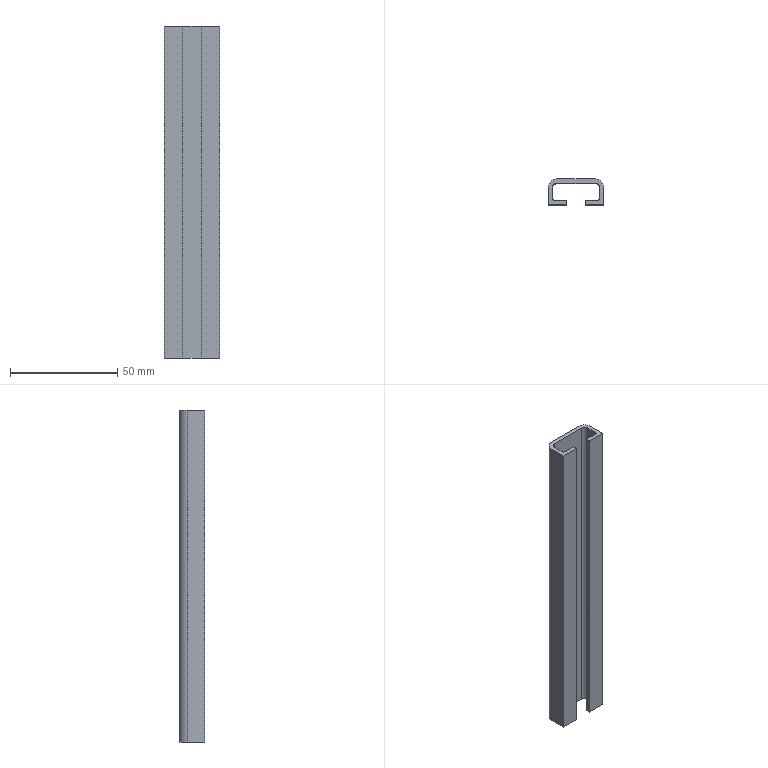Part | STEP file | V00-000000446 | 1 solid | 20 faces | box 26 x 12 x 155 mm | volume 17713 mm3 | plane 14 | cylinder 6 | commonest cylinder face diameters 2 x2 4 x2 8 x2
STEP:
#1=CARTESIAN_POINT('',(-4.25,0.,0.));
#2=VERTEX_POINT('',#1);
#3=CARTESIAN_POINT('',(-4.25,2.,0.));
#4=VERTEX_POINT('',#3);
#5=CARTESIAN_POINT('',(-4.25,1.,0.));
#6=DIRECTION('',(0.,1.,0.));
#7=VECTOR('',#6,1.);
#8=LINE('',#5,#7);
#9=EDGE_CURVE('',#2,#4,#8,.T.);
#10=ORIENTED_EDGE('',*,*,#9,.T.);
#11=CARTESIAN_POINT('',(-4.25,2.,155.));
#12=VERTEX_POINT('',#11);
#13=CARTESIAN_POINT('',(-4.25,2.,77.5));
#14=DIRECTION('',(0.,0.,-1.));
#15=VECTOR('',#14,1.);
#16=LINE('',#13,#15);
#17=EDGE_CURVE('',#12,#4,#16,.T.);
#18=ORIENTED_EDGE('',*,*,#17,.F.);
#19=CARTESIAN_POINT('',(-4.25,0.,155.));
#20=VERTEX_POINT('',#19);
#21=CARTESIAN_POINT('',(-4.25,1.,155.));
#22=DIRECTION('',(0.,1.,0.));
#23=VECTOR('',#22,1.);
#24=LINE('',#21,#23);
#25=EDGE_CURVE('',#20,#12,#24,.T.);
#26=ORIENTED_EDGE('',*,*,#25,.F.);
#27=CARTESIAN_POINT('',(-4.25,0.,77.5));
#28=DIRECTION('',(0.,0.,-1.));
#29=VECTOR('',#28,1.);
#30=LINE('',#27,#29);
#31=EDGE_CURVE('',#20,#2,#30,.T.);
#32=ORIENTED_EDGE('',*,*,#31,.T.);
#33=EDGE_LOOP('',(#10,#18,#26,#32));
#34=FACE_OUTER_BOUND('',#33,.T.);
#35=CARTESIAN_POINT('',(-4.25,2.,155.));
#36=DIRECTION('',(-1.,0.,0.));
#37=DIRECTION('',(0.,0.,1.));
#38=AXIS2_PLACEMENT_3D('',#35,#36,#37);
#39=PLANE('',#38);
#40=ADVANCED_FACE('',(#34),#39,.F.);
#41=ORIENTED_EDGE('',*,*,#9,.F.);
#42=CARTESIAN_POINT('',(-13.,0.,0.));
#43=VERTEX_POINT('',#42);
#44=CARTESIAN_POINT('',(-8.625,0.,0.));
#45=DIRECTION('',(1.,0.,0.));
#46=VECTOR('',#45,1.);
#47=LINE('',#44,#46);
#48=EDGE_CURVE('',#43,#2,#47,.T.);
#49=ORIENTED_EDGE('',*,*,#48,.F.);
#50=CARTESIAN_POINT('',(-13.,8.,0.));
#51=VERTEX_POINT('',#50);
#52=CARTESIAN_POINT('',(-13.,4.,0.));
#53=DIRECTION('',(0.,-1.,0.));
#54=VECTOR('',#53,1.);
#55=LINE('',#52,#54);
#56=EDGE_CURVE('',#51,#43,#55,.T.);
#57=ORIENTED_EDGE('',*,*,#56,.F.);
#58=CARTESIAN_POINT('',(-9.,12.,0.));
#59=VERTEX_POINT('',#58);
#60=CARTESIAN_POINT('',(-9.,8.,0.));
#61=DIRECTION('',(0.,0.,1.));
#62=AXIS2_PLACEMENT_3D('',#60,#61,$);
#63=CIRCLE('',#62,4.);
#64=EDGE_CURVE('',#59,#51,#63,.T.);
#65=ORIENTED_EDGE('',*,*,#64,.F.);
#66=CARTESIAN_POINT('',(9.,12.,0.));
#67=VERTEX_POINT('',#66);
#68=CARTESIAN_POINT('',(0.,12.,0.));
#69=DIRECTION('',(-1.,0.,0.));
#70=VECTOR('',#69,1.);
#71=LINE('',#68,#70);
#72=EDGE_CURVE('',#67,#59,#71,.T.);
#73=ORIENTED_EDGE('',*,*,#72,.F.);
#74=CARTESIAN_POINT('',(13.,8.,0.));
#75=VERTEX_POINT('',#74);
#76=CARTESIAN_POINT('',(9.,8.,0.));
#77=DIRECTION('',(0.,0.,1.));
#78=AXIS2_PLACEMENT_3D('',#76,#77,$);
#79=CIRCLE('',#78,4.);
#80=EDGE_CURVE('',#75,#67,#79,.T.);
#81=ORIENTED_EDGE('',*,*,#80,.F.);
#82=CARTESIAN_POINT('',(13.,0.,0.));
#83=VERTEX_POINT('',#82);
#84=CARTESIAN_POINT('',(13.,4.,0.));
#85=DIRECTION('',(0.,1.,0.));
#86=VECTOR('',#85,1.);
#87=LINE('',#84,#86);
#88=EDGE_CURVE('',#83,#75,#87,.T.);
#89=ORIENTED_EDGE('',*,*,#88,.F.);
#90=CARTESIAN_POINT('',(4.25,0.,0.));
#91=VERTEX_POINT('',#90);
#92=CARTESIAN_POINT('',(8.625,0.,0.));
#93=DIRECTION('',(1.,0.,0.));
#94=VECTOR('',#93,1.);
#95=LINE('',#92,#94);
#96=EDGE_CURVE('',#91,#83,#95,.T.);
#97=ORIENTED_EDGE('',*,*,#96,.F.);
#98=CARTESIAN_POINT('',(4.25,2.,0.));
#99=VERTEX_POINT('',#98);
#100=CARTESIAN_POINT('',(4.25,1.,0.));
#101=DIRECTION('',(0.,-1.,0.));
#102=VECTOR('',#101,1.);
#103=LINE('',#100,#102);
#104=EDGE_CURVE('',#99,#91,#103,.T.);
#105=ORIENTED_EDGE('',*,*,#104,.F.);
#106=CARTESIAN_POINT('',(10.,2.,0.));
#107=VERTEX_POINT('',#106);
#108=CARTESIAN_POINT('',(7.125,2.,0.));
#109=DIRECTION('',(-1.,0.,0.));
#110=VECTOR('',#109,1.);
#111=LINE('',#108,#110);
#112=EDGE_CURVE('',#107,#99,#111,.T.);
#113=ORIENTED_EDGE('',*,*,#112,.F.);
#114=CARTESIAN_POINT('',(11.,3.,0.));
#115=VERTEX_POINT('',#114);
#116=CARTESIAN_POINT('',(10.,3.,0.));
#117=DIRECTION('',(0.,0.,1.));
#118=AXIS2_PLACEMENT_3D('',#116,#117,$);
#119=CIRCLE('',#118,1.);
#120=EDGE_CURVE('',#107,#115,#119,.T.);
#121=ORIENTED_EDGE('',*,*,#120,.T.);
#122=CARTESIAN_POINT('',(11.,8.,0.));
#123=VERTEX_POINT('',#122);
#124=CARTESIAN_POINT('',(11.,5.5,0.));
#125=DIRECTION('',(0.,-1.,0.));
#126=VECTOR('',#125,1.);
#127=LINE('',#124,#126);
#128=EDGE_CURVE('',#123,#115,#127,.T.);
#129=ORIENTED_EDGE('',*,*,#128,.F.);
#130=CARTESIAN_POINT('',(9.,10.,0.));
#131=VERTEX_POINT('',#130);
#132=CARTESIAN_POINT('',(9.,10.,0.));
#133=CARTESIAN_POINT('',(9.208,10.,0.));
#134=CARTESIAN_POINT('',(9.416,9.973,0.));
#135=CARTESIAN_POINT('',(9.619,9.919,0.));
#136=CARTESIAN_POINT('',(10.006,9.759,0.));
#137=CARTESIAN_POINT('',(10.341,9.506,0.));
#138=CARTESIAN_POINT('',(10.49,9.358,0.));
#139=CARTESIAN_POINT('',(10.747,9.027,0.));
#140=CARTESIAN_POINT('',(10.911,8.642,0.));
#141=CARTESIAN_POINT('',(10.968,8.439,0.));
#142=CARTESIAN_POINT('',(10.998,8.227,0.));
#143=CARTESIAN_POINT('',(11.,8.014,0.));
#144=CARTESIAN_POINT('',(11.,8.01,0.));
#145=CARTESIAN_POINT('',(11.,8.005,0.));
#146=CARTESIAN_POINT('',(11.,8.,0.));
#147=B_SPLINE_CURVE_WITH_KNOTS('',5,(#132,#133,#134,#135,#136,#137,#138,#139,#140,#141,#142,#143,#144,#145,#146),.UNSPECIFIED.,.F.,.U.,(6,3,3,3,6),(0.,1.47,2.939,4.409,4.443),.UNSPECIFIED.);
#148=EDGE_CURVE('',#131,#123,#147,.T.);
#149=ORIENTED_EDGE('',*,*,#148,.F.);
#150=CARTESIAN_POINT('',(-9.,10.,0.));
#151=VERTEX_POINT('',#150);
#152=CARTESIAN_POINT('',(0.,10.,0.));
#153=DIRECTION('',(1.,0.,0.));
#154=VECTOR('',#153,1.);
#155=LINE('',#152,#154);
#156=EDGE_CURVE('',#151,#131,#155,.T.);
#157=ORIENTED_EDGE('',*,*,#156,.F.);
#158=CARTESIAN_POINT('',(-11.,8.,0.));
#159=VERTEX_POINT('',#158);
#160=CARTESIAN_POINT('',(-11.,8.,0.));
#161=CARTESIAN_POINT('',(-11.,8.208,0.));
#162=CARTESIAN_POINT('',(-10.973,8.416,0.));
#163=CARTESIAN_POINT('',(-10.919,8.619,0.));
#164=CARTESIAN_POINT('',(-10.759,9.006,0.));
#165=CARTESIAN_POINT('',(-10.506,9.341,0.));
#166=CARTESIAN_POINT('',(-10.358,9.49,0.));
#167=CARTESIAN_POINT('',(-10.027,9.747,0.));
#168=CARTESIAN_POINT('',(-9.642,9.911,0.));
#169=CARTESIAN_POINT('',(-9.439,9.968,0.));
#170=CARTESIAN_POINT('',(-9.227,9.998,0.));
#171=CARTESIAN_POINT('',(-9.014,10.,0.));
#172=CARTESIAN_POINT('',(-9.01,10.,0.));
#173=CARTESIAN_POINT('',(-9.005,10.,0.));
#174=CARTESIAN_POINT('',(-9.,10.,0.));
#175=B_SPLINE_CURVE_WITH_KNOTS('',5,(#160,#161,#162,#163,#164,#165,#166,#167,#168,#169,#170,#171,#172,#173,#174),.UNSPECIFIED.,.F.,.U.,(6,3,3,3,6),(0.,1.47,2.939,4.409,4.443),.UNSPECIFIED.);
#176=EDGE_CURVE('',#159,#151,#175,.T.);
#177=ORIENTED_EDGE('',*,*,#176,.F.);
#178=CARTESIAN_POINT('',(-11.,3.,0.));
#179=VERTEX_POINT('',#178);
#180=CARTESIAN_POINT('',(-11.,5.5,0.));
#181=DIRECTION('',(0.,1.,0.));
#182=VECTOR('',#181,1.);
#183=LINE('',#180,#182);
#184=EDGE_CURVE('',#179,#159,#183,.T.);
#185=ORIENTED_EDGE('',*,*,#184,.F.);
#186=CARTESIAN_POINT('',(-10.,2.,0.));
#187=VERTEX_POINT('',#186);
#188=CARTESIAN_POINT('',(-10.,3.,0.));
#189=DIRECTION('',(0.,0.,1.));
#190=AXIS2_PLACEMENT_3D('',#188,#189,$);
#191=CIRCLE('',#190,1.);
#192=EDGE_CURVE('',#179,#187,#191,.T.);
#193=ORIENTED_EDGE('',*,*,#192,.T.);
#194=CARTESIAN_POINT('',(-7.125,2.,0.));
#195=DIRECTION('',(-1.,0.,0.));
#196=VECTOR('',#195,1.);
#197=LINE('',#194,#196);
#198=EDGE_CURVE('',#4,#187,#197,.T.);
#199=ORIENTED_EDGE('',*,*,#198,.F.);
#200=EDGE_LOOP('',(#41,#49,#57,#65,#73,#81,#89,#97,#105,#113,#121,#129,#149,#157,#177,#185,#193,#199));
#201=FACE_OUTER_BOUND('',#200,.T.);
#202=CARTESIAN_POINT('',(-9.,8.,0.));
#203=DIRECTION('',(0.,0.,1.));
#204=DIRECTION('',(1.,0.,0.));
#205=AXIS2_PLACEMENT_3D('',#202,#203,#204);
#206=PLANE('',#205);
#207=ADVANCED_FACE('',(#201),#206,.F.);
#208=ORIENTED_EDGE('',*,*,#198,.T.);
#209=CARTESIAN_POINT('',(-10.,2.,155.));
#210=VERTEX_POINT('',#209);
#211=CARTESIAN_POINT('',(-10.,2.,77.5));
#212=DIRECTION('',(0.,0.,1.));
#213=VECTOR('',#212,1.);
#214=LINE('',#211,#213);
#215=EDGE_CURVE('',#187,#210,#214,.T.);
#216=ORIENTED_EDGE('',*,*,#215,.T.);
#217=CARTESIAN_POINT('',(-7.125,2.,155.));
#218=DIRECTION('',(-1.,0.,0.));
#219=VECTOR('',#218,1.);
#220=LINE('',#217,#219);
#221=EDGE_CURVE('',#12,#210,#220,.T.);
#222=ORIENTED_EDGE('',*,*,#221,.F.);
#223=ORIENTED_EDGE('',*,*,#17,.T.);
#224=EDGE_LOOP('',(#208,#216,#222,#223));
#225=FACE_OUTER_BOUND('',#224,.T.);
#226=CARTESIAN_POINT('',(-4.25,2.,155.));
#227=DIRECTION('',(0.,-1.,0.));
#228=DIRECTION('',(0.,0.,-1.));
#229=AXIS2_PLACEMENT_3D('',#226,#227,#228);
#230=PLANE('',#229);
#231=ADVANCED_FACE('',(#225),#230,.F.);
#232=ORIENTED_EDGE('',*,*,#25,.T.);
#233=ORIENTED_EDGE('',*,*,#221,.T.);
#234=CARTESIAN_POINT('',(-11.,3.,155.));
#235=VERTEX_POINT('',#234);
#236=CARTESIAN_POINT('',(-10.,2.,155.));
#237=CARTESIAN_POINT('',(-10.098,2.,155.));
#238=CARTESIAN_POINT('',(-10.196,2.012,155.));
#239=CARTESIAN_POINT('',(-10.292,2.036,155.));
#240=CARTESIAN_POINT('',(-10.476,2.107,155.));
#241=CARTESIAN_POINT('',(-10.638,2.22,155.));
#242=CARTESIAN_POINT('',(-10.711,2.287,155.));
#243=CARTESIAN_POINT('',(-10.84,2.436,155.));
#244=CARTESIAN_POINT('',(-10.93,2.612,155.));
#245=CARTESIAN_POINT('',(-10.963,2.705,155.));
#246=CARTESIAN_POINT('',(-10.99,2.821,155.));
#247=CARTESIAN_POINT('',(-10.998,2.939,155.));
#248=CARTESIAN_POINT('',(-10.999,2.96,155.));
#249=CARTESIAN_POINT('',(-11.,2.98,155.));
#250=CARTESIAN_POINT('',(-11.,3.,155.));
#251=B_SPLINE_CURVE_WITH_KNOTS('',5,(#236,#237,#238,#239,#240,#241,#242,#243,#244,#245,#246,#247,#248,#249,#250),.UNSPECIFIED.,.F.,.U.,(6,3,3,3,6),(0.,0.6928,1.386,2.078,2.221),.UNSPECIFIED.);
#252=EDGE_CURVE('',#210,#235,#251,.T.);
#253=ORIENTED_EDGE('',*,*,#252,.T.);
#254=CARTESIAN_POINT('',(-11.,8.,155.));
#255=VERTEX_POINT('',#254);
#256=CARTESIAN_POINT('',(-11.,5.5,155.));
#257=DIRECTION('',(0.,1.,0.));
#258=VECTOR('',#257,1.);
#259=LINE('',#256,#258);
#260=EDGE_CURVE('',#235,#255,#259,.T.);
#261=ORIENTED_EDGE('',*,*,#260,.T.);
#262=CARTESIAN_POINT('',(-9.,10.,155.));
#263=VERTEX_POINT('',#262);
#264=CARTESIAN_POINT('',(-11.,8.,155.));
#265=CARTESIAN_POINT('',(-11.,8.208,155.));
#266=CARTESIAN_POINT('',(-10.973,8.416,155.));
#267=CARTESIAN_POINT('',(-10.919,8.619,155.));
#268=CARTESIAN_POINT('',(-10.759,9.006,155.));
#269=CARTESIAN_POINT('',(-10.506,9.341,155.));
#270=CARTESIAN_POINT('',(-10.358,9.49,155.));
#271=CARTESIAN_POINT('',(-10.027,9.747,155.));
#272=CARTESIAN_POINT('',(-9.642,9.911,155.));
#273=CARTESIAN_POINT('',(-9.439,9.968,155.));
#274=CARTESIAN_POINT('',(-9.227,9.998,155.));
#275=CARTESIAN_POINT('',(-9.014,10.,155.));
#276=CARTESIAN_POINT('',(-9.01,10.,155.));
#277=CARTESIAN_POINT('',(-9.005,10.,155.));
#278=CARTESIAN_POINT('',(-9.,10.,155.));
#279=B_SPLINE_CURVE_WITH_KNOTS('',5,(#264,#265,#266,#267,#268,#269,#270,#271,#272,#273,#274,#275,#276,#277,#278),.UNSPECIFIED.,.F.,.U.,(6,3,3,3,6),(0.,1.47,2.939,4.409,4.443),.UNSPECIFIED.);
#280=EDGE_CURVE('',#255,#263,#279,.T.);
#281=ORIENTED_EDGE('',*,*,#280,.T.);
#282=CARTESIAN_POINT('',(9.,10.,155.));
#283=VERTEX_POINT('',#282);
#284=CARTESIAN_POINT('',(0.,10.,155.));
#285=DIRECTION('',(1.,0.,0.));
#286=VECTOR('',#285,1.);
#287=LINE('',#284,#286);
#288=EDGE_CURVE('',#263,#283,#287,.T.);
#289=ORIENTED_EDGE('',*,*,#288,.T.);
#290=CARTESIAN_POINT('',(11.,8.,155.));
#291=VERTEX_POINT('',#290);
#292=CARTESIAN_POINT('',(9.,10.,155.));
#293=CARTESIAN_POINT('',(9.208,10.,155.));
#294=CARTESIAN_POINT('',(9.416,9.973,155.));
#295=CARTESIAN_POINT('',(9.619,9.919,155.));
#296=CARTESIAN_POINT('',(10.006,9.759,155.));
#297=CARTESIAN_POINT('',(10.341,9.506,155.));
#298=CARTESIAN_POINT('',(10.49,9.358,155.));
#299=CARTESIAN_POINT('',(10.747,9.027,155.));
#300=CARTESIAN_POINT('',(10.911,8.642,155.));
#301=CARTESIAN_POINT('',(10.968,8.439,155.));
#302=CARTESIAN_POINT('',(10.998,8.227,155.));
#303=CARTESIAN_POINT('',(11.,8.014,155.));
#304=CARTESIAN_POINT('',(11.,8.01,155.));
#305=CARTESIAN_POINT('',(11.,8.005,155.));
#306=CARTESIAN_POINT('',(11.,8.,155.));
#307=B_SPLINE_CURVE_WITH_KNOTS('',5,(#292,#293,#294,#295,#296,#297,#298,#299,#300,#301,#302,#303,#304,#305,#306),.UNSPECIFIED.,.F.,.U.,(6,3,3,3,6),(0.,1.47,2.939,4.409,4.443),.UNSPECIFIED.);
#308=EDGE_CURVE('',#283,#291,#307,.T.);
#309=ORIENTED_EDGE('',*,*,#308,.T.);
#310=CARTESIAN_POINT('',(11.,3.,155.));
#311=VERTEX_POINT('',#310);
#312=CARTESIAN_POINT('',(11.,5.5,155.));
#313=DIRECTION('',(0.,-1.,0.));
#314=VECTOR('',#313,1.);
#315=LINE('',#312,#314);
#316=EDGE_CURVE('',#291,#311,#315,.T.);
#317=ORIENTED_EDGE('',*,*,#316,.T.);
#318=CARTESIAN_POINT('',(10.,2.,155.));
#319=VERTEX_POINT('',#318);
#320=CARTESIAN_POINT('',(11.,3.,155.));
#321=CARTESIAN_POINT('',(11.,2.902,155.));
#322=CARTESIAN_POINT('',(10.988,2.804,155.));
#323=CARTESIAN_POINT('',(10.964,2.708,155.));
#324=CARTESIAN_POINT('',(10.893,2.524,155.));
#325=CARTESIAN_POINT('',(10.78,2.362,155.));
#326=CARTESIAN_POINT('',(10.713,2.289,155.));
#327=CARTESIAN_POINT('',(10.564,2.16,155.));
#328=CARTESIAN_POINT('',(10.388,2.07,155.));
#329=CARTESIAN_POINT('',(10.295,2.037,155.));
#330=CARTESIAN_POINT('',(10.179,2.01,155.));
#331=CARTESIAN_POINT('',(10.061,2.002,155.));
#332=CARTESIAN_POINT('',(10.04,2.001,155.));
#333=CARTESIAN_POINT('',(10.02,2.,155.));
#334=CARTESIAN_POINT('',(10.,2.,155.));
#335=B_SPLINE_CURVE_WITH_KNOTS('',5,(#320,#321,#322,#323,#324,#325,#326,#327,#328,#329,#330,#331,#332,#333,#334),.UNSPECIFIED.,.F.,.U.,(6,3,3,3,6),(0.,0.6928,1.386,2.078,2.221),.UNSPECIFIED.);
#336=EDGE_CURVE('',#311,#319,#335,.T.);
#337=ORIENTED_EDGE('',*,*,#336,.T.);
#338=CARTESIAN_POINT('',(4.25,2.,155.));
#339=VERTEX_POINT('',#338);
#340=CARTESIAN_POINT('',(7.125,2.,155.));
#341=DIRECTION('',(-1.,0.,0.));
#342=VECTOR('',#341,1.);
#343=LINE('',#340,#342);
#344=EDGE_CURVE('',#319,#339,#343,.T.);
#345=ORIENTED_EDGE('',*,*,#344,.T.);
#346=CARTESIAN_POINT('',(4.25,0.,155.));
#347=VERTEX_POINT('',#346);
#348=CARTESIAN_POINT('',(4.25,1.,155.));
#349=DIRECTION('',(0.,-1.,0.));
#350=VECTOR('',#349,1.);
#351=LINE('',#348,#350);
#352=EDGE_CURVE('',#339,#347,#351,.T.);
#353=ORIENTED_EDGE('',*,*,#352,.T.);
#354=CARTESIAN_POINT('',(13.,0.,155.));
#355=VERTEX_POINT('',#354);
#356=CARTESIAN_POINT('',(8.625,0.,155.));
#357=DIRECTION('',(1.,0.,0.));
#358=VECTOR('',#357,1.);
#359=LINE('',#356,#358);
#360=EDGE_CURVE('',#347,#355,#359,.T.);
#361=ORIENTED_EDGE('',*,*,#360,.T.);
#362=CARTESIAN_POINT('',(13.,8.,155.));
#363=VERTEX_POINT('',#362);
#364=CARTESIAN_POINT('',(13.,4.,155.));
#365=DIRECTION('',(0.,1.,0.));
#366=VECTOR('',#365,1.);
#367=LINE('',#364,#366);
#368=EDGE_CURVE('',#355,#363,#367,.T.);
#369=ORIENTED_EDGE('',*,*,#368,.T.);
#370=CARTESIAN_POINT('',(9.,12.,155.));
#371=VERTEX_POINT('',#370);
#372=CARTESIAN_POINT('',(9.,8.,155.));
#373=DIRECTION('',(0.,0.,1.));
#374=AXIS2_PLACEMENT_3D('',#372,#373,$);
#375=CIRCLE('',#374,4.);
#376=EDGE_CURVE('',#363,#371,#375,.T.);
#377=ORIENTED_EDGE('',*,*,#376,.T.);
#378=CARTESIAN_POINT('',(-9.,12.,155.));
#379=VERTEX_POINT('',#378);
#380=CARTESIAN_POINT('',(0.,12.,155.));
#381=DIRECTION('',(-1.,0.,0.));
#382=VECTOR('',#381,1.);
#383=LINE('',#380,#382);
#384=EDGE_CURVE('',#371,#379,#383,.T.);
#385=ORIENTED_EDGE('',*,*,#384,.T.);
#386=CARTESIAN_POINT('',(-13.,8.,155.));
#387=VERTEX_POINT('',#386);
#388=CARTESIAN_POINT('',(-9.,8.,155.));
#389=DIRECTION('',(0.,0.,1.));
#390=AXIS2_PLACEMENT_3D('',#388,#389,$);
#391=CIRCLE('',#390,4.);
#392=EDGE_CURVE('',#379,#387,#391,.T.);
#393=ORIENTED_EDGE('',*,*,#392,.T.);
#394=CARTESIAN_POINT('',(-13.,0.,155.));
#395=VERTEX_POINT('',#394);
#396=CARTESIAN_POINT('',(-13.,4.,155.));
#397=DIRECTION('',(0.,-1.,0.));
#398=VECTOR('',#397,1.);
#399=LINE('',#396,#398);
#400=EDGE_CURVE('',#387,#395,#399,.T.);
#401=ORIENTED_EDGE('',*,*,#400,.T.);
#402=CARTESIAN_POINT('',(-8.625,0.,155.));
#403=DIRECTION('',(1.,0.,0.));
#404=VECTOR('',#403,1.);
#405=LINE('',#402,#404);
#406=EDGE_CURVE('',#395,#20,#405,.T.);
#407=ORIENTED_EDGE('',*,*,#406,.T.);
#408=EDGE_LOOP('',(#232,#233,#253,#261,#281,#289,#309,#317,#337,#345,#353,#361,#369,#377,#385,#393,#401,#407));
#409=FACE_OUTER_BOUND('',#408,.T.);
#410=CARTESIAN_POINT('',(-9.,8.,155.));
#411=DIRECTION('',(0.,0.,1.));
#412=DIRECTION('',(1.,0.,0.));
#413=AXIS2_PLACEMENT_3D('',#410,#411,#412);
#414=PLANE('',#413);
#415=ADVANCED_FACE('',(#409),#414,.T.);
#416=ORIENTED_EDGE('',*,*,#48,.T.);
#417=ORIENTED_EDGE('',*,*,#31,.F.);
#418=ORIENTED_EDGE('',*,*,#406,.F.);
#419=CARTESIAN_POINT('',(-13.,0.,77.5));
#420=DIRECTION('',(0.,0.,-1.));
#421=VECTOR('',#420,1.);
#422=LINE('',#419,#421);
#423=EDGE_CURVE('',#395,#43,#422,.T.);
#424=ORIENTED_EDGE('',*,*,#423,.T.);
#425=EDGE_LOOP('',(#416,#417,#418,#424));
#426=FACE_OUTER_BOUND('',#425,.T.);
#427=CARTESIAN_POINT('',(-4.25,0.,155.));
#428=DIRECTION('',(0.,1.,0.));
#429=DIRECTION('',(-1.,0.,0.));
#430=AXIS2_PLACEMENT_3D('',#427,#428,#429);
#431=PLANE('',#430);
#432=ADVANCED_FACE('',(#426),#431,.F.);
#433=ORIENTED_EDGE('',*,*,#56,.T.);
#434=ORIENTED_EDGE('',*,*,#423,.F.);
#435=ORIENTED_EDGE('',*,*,#400,.F.);
#436=CARTESIAN_POINT('',(-13.,8.,77.5));
#437=DIRECTION('',(0.,0.,-1.));
#438=VECTOR('',#437,1.);
#439=LINE('',#436,#438);
#440=EDGE_CURVE('',#387,#51,#439,.T.);
#441=ORIENTED_EDGE('',*,*,#440,.T.);
#442=EDGE_LOOP('',(#433,#434,#435,#441));
#443=FACE_OUTER_BOUND('',#442,.T.);
#444=CARTESIAN_POINT('',(-13.,0.,155.));
#445=DIRECTION('',(1.,0.,0.));
#446=DIRECTION('',(0.,0.,-1.));
#447=AXIS2_PLACEMENT_3D('',#444,#445,#446);
#448=PLANE('',#447);
#449=ADVANCED_FACE('',(#443),#448,.F.);
#450=ORIENTED_EDGE('',*,*,#64,.T.);
#451=ORIENTED_EDGE('',*,*,#440,.F.);
#452=ORIENTED_EDGE('',*,*,#392,.F.);
#453=CARTESIAN_POINT('',(-9.,12.,155.));
#454=DIRECTION('',(0.,0.,-1.));
#455=VECTOR('',#454,1.);
#456=LINE('',#453,#455);
#457=EDGE_CURVE('',#379,#59,#456,.T.);
#458=ORIENTED_EDGE('',*,*,#457,.T.);
#459=EDGE_LOOP('',(#450,#451,#452,#458));
#460=FACE_OUTER_BOUND('',#459,.T.);
#461=CARTESIAN_POINT('',(-9.,8.,155.));
#462=DIRECTION('',(0.,0.,-1.));
#463=DIRECTION('',(-1.,0.,0.));
#464=AXIS2_PLACEMENT_3D('',#461,#462,#463);
#465=CYLINDRICAL_SURFACE('',#464,4.);
#466=ADVANCED_FACE('',(#460),#465,.T.);
#467=ORIENTED_EDGE('',*,*,#72,.T.);
#468=ORIENTED_EDGE('',*,*,#457,.F.);
#469=ORIENTED_EDGE('',*,*,#384,.F.);
#470=CARTESIAN_POINT('',(9.,12.,77.5));
#471=DIRECTION('',(0.,0.,-1.));
#472=VECTOR('',#471,1.);
#473=LINE('',#470,#472);
#474=EDGE_CURVE('',#371,#67,#473,.T.);
#475=ORIENTED_EDGE('',*,*,#474,.T.);
#476=EDGE_LOOP('',(#467,#468,#469,#475));
#477=FACE_OUTER_BOUND('',#476,.T.);
#478=CARTESIAN_POINT('',(-9.,12.,155.));
#479=DIRECTION('',(0.,-1.,0.));
#480=DIRECTION('',(0.,0.,-1.));
#481=AXIS2_PLACEMENT_3D('',#478,#479,#480);
#482=PLANE('',#481);
#483=ADVANCED_FACE('',(#477),#482,.F.);
#484=ORIENTED_EDGE('',*,*,#80,.T.);
#485=ORIENTED_EDGE('',*,*,#474,.F.);
#486=ORIENTED_EDGE('',*,*,#376,.F.);
#487=CARTESIAN_POINT('',(13.,8.,155.));
#488=DIRECTION('',(0.,0.,-1.));
#489=VECTOR('',#488,1.);
#490=LINE('',#487,#489);
#491=EDGE_CURVE('',#363,#75,#490,.T.);
#492=ORIENTED_EDGE('',*,*,#491,.T.);
#493=EDGE_LOOP('',(#484,#485,#486,#492));
#494=FACE_OUTER_BOUND('',#493,.T.);
#495=CARTESIAN_POINT('',(9.,8.,155.));
#496=DIRECTION('',(0.,0.,-1.));
#497=DIRECTION('',(-1.,0.,0.));
#498=AXIS2_PLACEMENT_3D('',#495,#496,#497);
#499=CYLINDRICAL_SURFACE('',#498,4.);
#500=ADVANCED_FACE('',(#494),#499,.T.);
#501=ORIENTED_EDGE('',*,*,#88,.T.);
#502=ORIENTED_EDGE('',*,*,#491,.F.);
#503=ORIENTED_EDGE('',*,*,#368,.F.);
#504=CARTESIAN_POINT('',(13.,0.,77.5));
#505=DIRECTION('',(0.,0.,-1.));
#506=VECTOR('',#505,1.);
#507=LINE('',#504,#506);
#508=EDGE_CURVE('',#355,#83,#507,.T.);
#509=ORIENTED_EDGE('',*,*,#508,.T.);
#510=EDGE_LOOP('',(#501,#502,#503,#509));
#511=FACE_OUTER_BOUND('',#510,.T.);
#512=CARTESIAN_POINT('',(13.,0.,155.));
#513=DIRECTION('',(-1.,0.,0.));
#514=DIRECTION('',(0.,0.,1.));
#515=AXIS2_PLACEMENT_3D('',#512,#513,#514);
#516=PLANE('',#515);
#517=ADVANCED_FACE('',(#511),#516,.F.);
#518=ORIENTED_EDGE('',*,*,#96,.T.);
#519=ORIENTED_EDGE('',*,*,#508,.F.);
#520=ORIENTED_EDGE('',*,*,#360,.F.);
#521=CARTESIAN_POINT('',(4.25,0.,77.5));
#522=DIRECTION('',(0.,0.,-1.));
#523=VECTOR('',#522,1.);
#524=LINE('',#521,#523);
#525=EDGE_CURVE('',#347,#91,#524,.T.);
#526=ORIENTED_EDGE('',*,*,#525,.T.);
#527=EDGE_LOOP('',(#518,#519,#520,#526));
#528=FACE_OUTER_BOUND('',#527,.T.);
#529=CARTESIAN_POINT('',(4.25,0.,155.));
#530=DIRECTION('',(0.,1.,0.));
#531=DIRECTION('',(-1.,0.,0.));
#532=AXIS2_PLACEMENT_3D('',#529,#530,#531);
#533=PLANE('',#532);
#534=ADVANCED_FACE('',(#528),#533,.F.);
#535=ORIENTED_EDGE('',*,*,#104,.T.);
#536=ORIENTED_EDGE('',*,*,#525,.F.);
#537=ORIENTED_EDGE('',*,*,#352,.F.);
#538=CARTESIAN_POINT('',(4.25,2.,77.5));
#539=DIRECTION('',(0.,0.,-1.));
#540=VECTOR('',#539,1.);
#541=LINE('',#538,#540);
#542=EDGE_CURVE('',#339,#99,#541,.T.);
#543=ORIENTED_EDGE('',*,*,#542,.T.);
#544=EDGE_LOOP('',(#535,#536,#537,#543));
#545=FACE_OUTER_BOUND('',#544,.T.);
#546=CARTESIAN_POINT('',(4.25,2.,155.));
#547=DIRECTION('',(1.,0.,0.));
#548=DIRECTION('',(0.,0.,-1.));
#549=AXIS2_PLACEMENT_3D('',#546,#547,#548);
#550=PLANE('',#549);
#551=ADVANCED_FACE('',(#545),#550,.F.);
#552=ORIENTED_EDGE('',*,*,#344,.F.);
#553=CARTESIAN_POINT('',(10.,2.,77.5));
#554=DIRECTION('',(0.,0.,-1.));
#555=VECTOR('',#554,1.);
#556=LINE('',#553,#555);
#557=EDGE_CURVE('',#319,#107,#556,.T.);
#558=ORIENTED_EDGE('',*,*,#557,.T.);
#559=ORIENTED_EDGE('',*,*,#112,.T.);
#560=ORIENTED_EDGE('',*,*,#542,.F.);
#561=EDGE_LOOP('',(#552,#558,#559,#560));
#562=FACE_OUTER_BOUND('',#561,.T.);
#563=CARTESIAN_POINT('',(4.25,2.,155.));
#564=DIRECTION('',(0.,-1.,0.));
#565=DIRECTION('',(0.,0.,-1.));
#566=AXIS2_PLACEMENT_3D('',#563,#564,#565);
#567=PLANE('',#566);
#568=ADVANCED_FACE('',(#562),#567,.F.);
#569=ORIENTED_EDGE('',*,*,#336,.F.);
#570=CARTESIAN_POINT('',(11.,3.,155.));
#571=DIRECTION('',(0.,0.,1.));
#572=VECTOR('',#571,1.);
#573=LINE('',#570,#572);
#574=EDGE_CURVE('',#115,#311,#573,.T.);
#575=ORIENTED_EDGE('',*,*,#574,.F.);
#576=ORIENTED_EDGE('',*,*,#120,.F.);
#577=ORIENTED_EDGE('',*,*,#557,.F.);
#578=EDGE_LOOP('',(#569,#575,#576,#577));
#579=FACE_OUTER_BOUND('',#578,.T.);
#580=CARTESIAN_POINT('',(10.,3.,155.));
#581=DIRECTION('',(0.,0.,1.));
#582=DIRECTION('',(-1.,0.,0.));
#583=AXIS2_PLACEMENT_3D('',#580,#581,#582);
#584=CYLINDRICAL_SURFACE('',#583,1.);
#585=ADVANCED_FACE('',(#579),#584,.F.);
#586=ORIENTED_EDGE('',*,*,#128,.T.);
#587=ORIENTED_EDGE('',*,*,#574,.T.);
#588=ORIENTED_EDGE('',*,*,#316,.F.);
#589=CARTESIAN_POINT('',(11.,8.,77.5));
#590=DIRECTION('',(0.,0.,-1.));
#591=VECTOR('',#590,1.);
#592=LINE('',#589,#591);
#593=EDGE_CURVE('',#291,#123,#592,.T.);
#594=ORIENTED_EDGE('',*,*,#593,.T.);
#595=EDGE_LOOP('',(#586,#587,#588,#594));
#596=FACE_OUTER_BOUND('',#595,.T.);
#597=CARTESIAN_POINT('',(11.,2.,155.));
#598=DIRECTION('',(1.,0.,0.));
#599=DIRECTION('',(0.,0.,-1.));
#600=AXIS2_PLACEMENT_3D('',#597,#598,#599);
#601=PLANE('',#600);
#602=ADVANCED_FACE('',(#596),#601,.F.);
#603=ORIENTED_EDGE('',*,*,#148,.T.);
#604=ORIENTED_EDGE('',*,*,#593,.F.);
#605=ORIENTED_EDGE('',*,*,#308,.F.);
#606=CARTESIAN_POINT('',(9.,10.,155.));
#607=DIRECTION('',(0.,0.,-1.));
#608=VECTOR('',#607,1.);
#609=LINE('',#606,#608);
#610=EDGE_CURVE('',#283,#131,#609,.T.);
#611=ORIENTED_EDGE('',*,*,#610,.T.);
#612=EDGE_LOOP('',(#603,#604,#605,#611));
#613=FACE_OUTER_BOUND('',#612,.T.);
#614=CARTESIAN_POINT('',(9.,8.,155.));
#615=DIRECTION('',(0.,0.,-1.));
#616=DIRECTION('',(-1.,0.,0.));
#617=AXIS2_PLACEMENT_3D('',#614,#615,#616);
#618=CYLINDRICAL_SURFACE('',#617,2.);
#619=ADVANCED_FACE('',(#613),#618,.F.);
#620=ORIENTED_EDGE('',*,*,#156,.T.);
#621=ORIENTED_EDGE('',*,*,#610,.F.);
#622=ORIENTED_EDGE('',*,*,#288,.F.);
#623=CARTESIAN_POINT('',(-9.,10.,77.5));
#624=DIRECTION('',(0.,0.,-1.));
#625=VECTOR('',#624,1.);
#626=LINE('',#623,#625);
#627=EDGE_CURVE('',#263,#151,#626,.T.);
#628=ORIENTED_EDGE('',*,*,#627,.T.);
#629=EDGE_LOOP('',(#620,#621,#622,#628));
#630=FACE_OUTER_BOUND('',#629,.T.);
#631=CARTESIAN_POINT('',(-9.,10.,155.));
#632=DIRECTION('',(0.,1.,0.));
#633=DIRECTION('',(0.,0.,1.));
#634=AXIS2_PLACEMENT_3D('',#631,#632,#633);
#635=PLANE('',#634);
#636=ADVANCED_FACE('',(#630),#635,.F.);
#637=ORIENTED_EDGE('',*,*,#176,.T.);
#638=ORIENTED_EDGE('',*,*,#627,.F.);
#639=ORIENTED_EDGE('',*,*,#280,.F.);
#640=CARTESIAN_POINT('',(-11.,8.,155.));
#641=DIRECTION('',(0.,0.,-1.));
#642=VECTOR('',#641,1.);
#643=LINE('',#640,#642);
#644=EDGE_CURVE('',#255,#159,#643,.T.);
#645=ORIENTED_EDGE('',*,*,#644,.T.);
#646=EDGE_LOOP('',(#637,#638,#639,#645));
#647=FACE_OUTER_BOUND('',#646,.T.);
#648=CARTESIAN_POINT('',(-9.,8.,155.));
#649=DIRECTION('',(0.,0.,-1.));
#650=DIRECTION('',(-1.,0.,0.));
#651=AXIS2_PLACEMENT_3D('',#648,#649,#650);
#652=CYLINDRICAL_SURFACE('',#651,2.);
#653=ADVANCED_FACE('',(#647),#652,.F.);
#654=ORIENTED_EDGE('',*,*,#260,.F.);
#655=CARTESIAN_POINT('',(-11.,3.,77.5));
#656=DIRECTION('',(0.,0.,-1.));
#657=VECTOR('',#656,1.);
#658=LINE('',#655,#657);
#659=EDGE_CURVE('',#235,#179,#658,.T.);
#660=ORIENTED_EDGE('',*,*,#659,.T.);
#661=ORIENTED_EDGE('',*,*,#184,.T.);
#662=ORIENTED_EDGE('',*,*,#644,.F.);
#663=EDGE_LOOP('',(#654,#660,#661,#662));
#664=FACE_OUTER_BOUND('',#663,.T.);
#665=CARTESIAN_POINT('',(-11.,2.,155.));
#666=DIRECTION('',(-1.,0.,0.));
#667=DIRECTION('',(0.,-1.,0.));
#668=AXIS2_PLACEMENT_3D('',#665,#666,#667);
#669=PLANE('',#668);
#670=ADVANCED_FACE('',(#664),#669,.F.);
#671=ORIENTED_EDGE('',*,*,#252,.F.);
#672=ORIENTED_EDGE('',*,*,#215,.F.);
#673=ORIENTED_EDGE('',*,*,#192,.F.);
#674=ORIENTED_EDGE('',*,*,#659,.F.);
#675=EDGE_LOOP('',(#671,#672,#673,#674));
#676=FACE_OUTER_BOUND('',#675,.T.);
#677=CARTESIAN_POINT('',(-10.,3.,155.));
#678=DIRECTION('',(0.,0.,1.));
#679=DIRECTION('',(-1.,0.,0.));
#680=AXIS2_PLACEMENT_3D('',#677,#678,#679);
#681=CYLINDRICAL_SURFACE('',#680,1.);
#682=ADVANCED_FACE('',(#676),#681,.F.);
#683=CLOSED_SHELL('',(#40,#207,#231,#415,#432,#449,#466,#483,#500,#517,#534,#551,#568,#585,#602,#619,#636,#653,#670,#682));
#684=MANIFOLD_SOLID_BREP('',#683);
#685=(LENGTH_UNIT()NAMED_UNIT(*)SI_UNIT(.MILLI.,.METRE.));
#686=UNCERTAINTY_MEASURE_WITH_UNIT(LENGTH_MEASURE(0.005),#685,'','');
#687=(NAMED_UNIT(*)PLANE_ANGLE_UNIT()SI_UNIT($,.RADIAN.));
#688=(NAMED_UNIT(*)SI_UNIT($,.STERADIAN.)SOLID_ANGLE_UNIT());
#689=(GEOMETRIC_REPRESENTATION_CONTEXT(3)GLOBAL_UNCERTAINTY_ASSIGNED_CONTEXT((#686))GLOBAL_UNIT_ASSIGNED_CONTEXT((#685,#687,#688))REPRESENTATION_CONTEXT('',''));
#690=ADVANCED_BREP_SHAPE_REPRESENTATION('',(#684),#689);